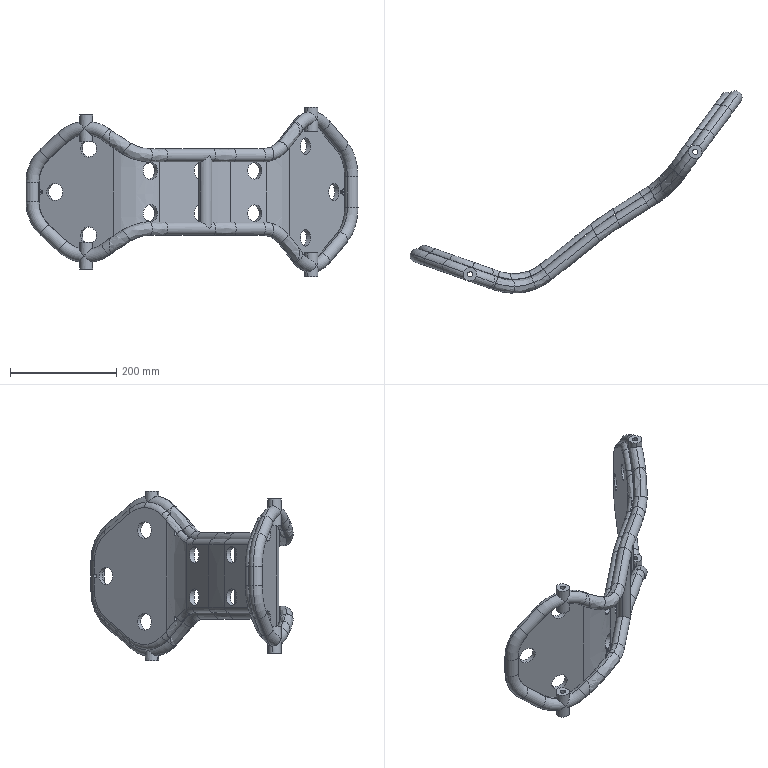Part | STEP file | Frame | 2 solids | 254 faces | box 624.751 x 380.553 x 318.558 mm | volume 2183546 mm3 | cylinder 96 | spline 82 | torus 48 | plane 28 | commonest cylinder face diameters 25 x44 32 x20 20 x14 10 x8 7 x6 3 x4